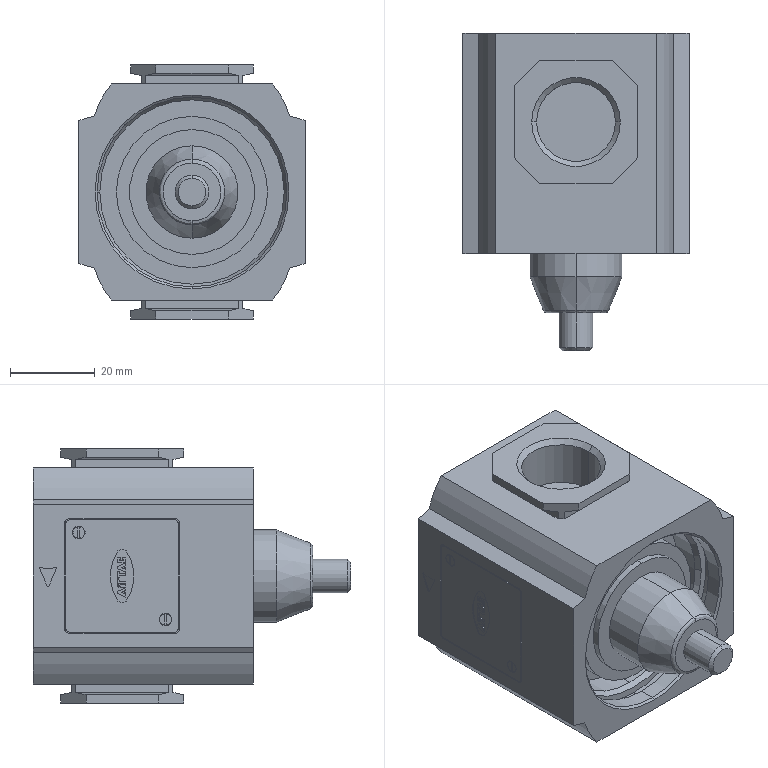Part | STEP file | Copy 2^GFC30015-A-F1 | 1 solid | 255 faces | box 53.4 x 75 x 60 mm | volume 121843 mm3 | plane 144 | cylinder 95 | cone 12 | spline 4 | commonest cylinder face diameters 2 x8 3 x8 4 x8 0.4 x7 0.488 x6 0.543 x5